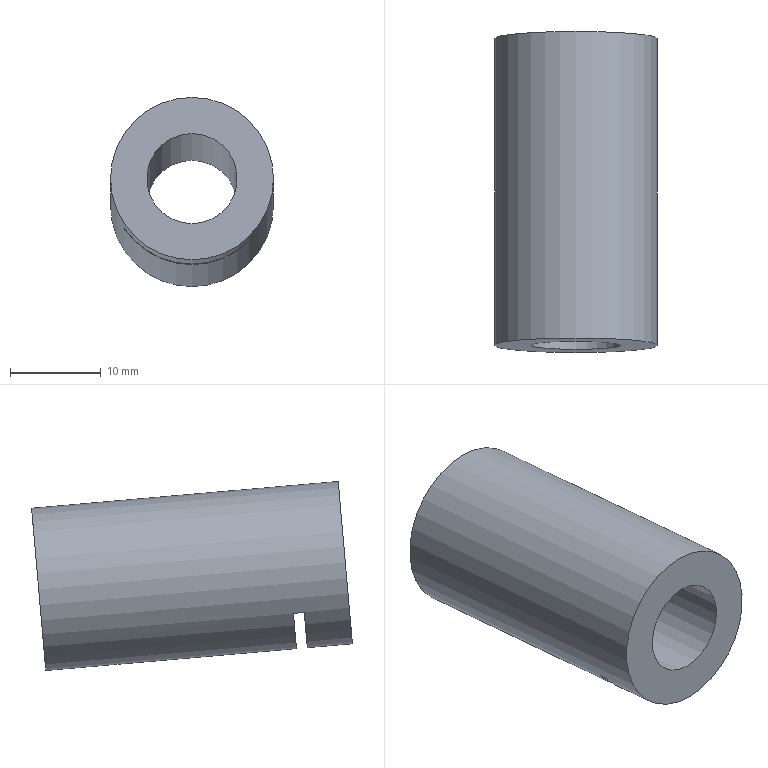Part | NX | features solid 2 | 1 solid | 7 faces | box 18 x 35.439 x 20.895 mm | volume 5933 mm3 | plane 5 | cylinder 2 | commonest cylinder face diameters 10 x1 18 x1
STEP:
#1=CARTESIAN_POINT('',(280.775,-80.843,-42.851));
#2=VERTEX_POINT('',#1);
#3=CARTESIAN_POINT('',(280.775,-81.278,-47.832));
#4=DIRECTION('',(0.,0.9962,-0.08716));
#5=DIRECTION('',(0.,0.08716,0.9962));
#6=AXIS2_PLACEMENT_3D('',#3,#4,#5);
#7=CIRCLE('',#6,5.);
#8=EDGE_CURVE('',#2,#2,#7,.T.);
#9=ORIENTED_EDGE('',*,*,#8,.F.);
#10=EDGE_LOOP('',(#9));
#11=FACE_BOUND('',#10,.T.);
#12=CARTESIAN_POINT('',(280.775,-80.494,-38.866));
#13=VERTEX_POINT('',#12);
#14=CARTESIAN_POINT('',(280.775,-81.278,-47.832));
#15=DIRECTION('',(0.,0.9962,-0.08716));
#16=DIRECTION('',(0.,0.08716,0.9962));
#17=AXIS2_PLACEMENT_3D('',#14,#15,#16);
#18=CIRCLE('',#17,9.);
#19=EDGE_CURVE('',#13,#13,#18,.F.);
#20=ORIENTED_EDGE('',*,*,#19,.F.);
#21=EDGE_LOOP('',(#20));
#22=FACE_BOUND('',#21,.T.);
#23=CARTESIAN_POINT('',(280.775,-81.278,-47.832));
#24=DIRECTION('',(0.,0.9962,-0.08716));
#25=DIRECTION('',(-1.,0.,0.));
#26=AXIS2_PLACEMENT_3D('',#23,#24,#25);
#27=PLANE('',#26);
#28=ADVANCED_FACE('',(#11,#22),#27,.T.);
#29=CARTESIAN_POINT('',(273.36,-110.612,-50.385));
#30=VERTEX_POINT('',#29);
#31=CARTESIAN_POINT('',(273.36,-109.417,-50.489));
#32=VERTEX_POINT('',#31);
#33=CARTESIAN_POINT('',(273.36,-57.017,-55.074));
#34=DIRECTION('',(0.,-0.9962,0.08716));
#35=VECTOR('',#34,1000.);
#36=LINE('',#33,#35);
#37=EDGE_CURVE('',#30,#32,#36,.F.);
#38=ORIENTED_EDGE('',*,*,#37,.F.);
#39=CARTESIAN_POINT('',(288.191,-110.612,-50.385));
#40=VERTEX_POINT('',#39);
#41=CARTESIAN_POINT('',(280.775,-110.168,-45.304));
#42=DIRECTION('',(0.,-0.9962,0.08716));
#43=DIRECTION('',(0.,-0.08716,-0.9962));
#44=AXIS2_PLACEMENT_3D('',#41,#42,#43);
#45=CIRCLE('',#44,9.);
#46=EDGE_CURVE('',#40,#30,#45,.F.);
#47=ORIENTED_EDGE('',*,*,#46,.F.);
#48=CARTESIAN_POINT('',(288.191,-109.417,-50.489));
#49=VERTEX_POINT('',#48);
#50=CARTESIAN_POINT('',(288.191,-57.017,-55.074));
#51=DIRECTION('',(0.,-0.9962,0.08716));
#52=VECTOR('',#51,1000.);
#53=LINE('',#50,#52);
#54=EDGE_CURVE('',#49,#40,#53,.T.);
#55=ORIENTED_EDGE('',*,*,#54,.F.);
#56=CARTESIAN_POINT('',(280.775,-108.973,-45.409));
#57=DIRECTION('',(0.,-0.9962,0.08716));
#58=DIRECTION('',(0.,-0.08716,-0.9962));
#59=AXIS2_PLACEMENT_3D('',#56,#57,#58);
#60=CIRCLE('',#59,9.);
#61=EDGE_CURVE('',#49,#32,#60,.F.);
#62=ORIENTED_EDGE('',*,*,#61,.T.);
#63=EDGE_LOOP('',(#38,#47,#55,#62));
#64=FACE_BOUND('',#63,.T.);
#65=ORIENTED_EDGE('',*,*,#19,.T.);
#66=EDGE_LOOP('',(#65));
#67=FACE_BOUND('',#66,.T.);
#68=CARTESIAN_POINT('',(280.775,-115.933,-53.834));
#69=VERTEX_POINT('',#68);
#70=CARTESIAN_POINT('',(280.775,-115.149,-44.868));
#71=DIRECTION('',(0.,-0.9962,0.08716));
#72=DIRECTION('',(0.,-0.08716,-0.9962));
#73=AXIS2_PLACEMENT_3D('',#70,#71,#72);
#74=CIRCLE('',#73,9.);
#75=EDGE_CURVE('',#69,#69,#74,.F.);
#76=ORIENTED_EDGE('',*,*,#75,.T.);
#77=EDGE_LOOP('',(#76));
#78=FACE_BOUND('',#77,.T.);
#79=CARTESIAN_POINT('',(280.775,-56.573,-49.993));
#80=DIRECTION('',(0.,-0.9962,0.08716));
#81=DIRECTION('',(1.,0.,0.));
#82=AXIS2_PLACEMENT_3D('',#79,#80,#81);
#83=CYLINDRICAL_SURFACE('',#82,9.);
#84=ADVANCED_FACE('',(#64,#67,#78),#83,.T.);
#85=CARTESIAN_POINT('',(280.775,-115.585,-49.849));
#86=VERTEX_POINT('',#85);
#87=CARTESIAN_POINT('',(280.775,-115.149,-44.868));
#88=DIRECTION('',(0.,-0.9962,0.08716));
#89=DIRECTION('',(0.,-0.08716,-0.9962));
#90=AXIS2_PLACEMENT_3D('',#87,#88,#89);
#91=CIRCLE('',#90,5.);
#92=EDGE_CURVE('',#86,#86,#91,.F.);
#93=ORIENTED_EDGE('',*,*,#92,.T.);
#94=EDGE_LOOP('',(#93));
#95=FACE_BOUND('',#94,.T.);
#96=ORIENTED_EDGE('',*,*,#75,.F.);
#97=EDGE_LOOP('',(#96));
#98=FACE_BOUND('',#97,.T.);
#99=CARTESIAN_POINT('',(280.775,-115.149,-44.868));
#100=DIRECTION('',(0.,-0.9962,0.08716));
#101=DIRECTION('',(-1.,0.,0.));
#102=AXIS2_PLACEMENT_3D('',#99,#100,#101);
#103=PLANE('',#102);
#104=ADVANCED_FACE('',(#95,#98),#103,.T.);
#105=ORIENTED_EDGE('',*,*,#8,.T.);
#106=EDGE_LOOP('',(#105));
#107=FACE_BOUND('',#106,.T.);
#108=ORIENTED_EDGE('',*,*,#92,.F.);
#109=EDGE_LOOP('',(#108));
#110=FACE_BOUND('',#109,.T.);
#111=CARTESIAN_POINT('',(280.775,-73.508,-48.512));
#112=DIRECTION('',(0.,-0.9962,0.08716));
#113=DIRECTION('',(0.,-0.08716,-0.9962));
#114=AXIS2_PLACEMENT_3D('',#111,#112,#113);
#115=CYLINDRICAL_SURFACE('',#114,5.);
#116=ADVANCED_FACE('',(#107,#110),#115,.F.);
#117=CARTESIAN_POINT('',(273.292,-109.417,-50.489));
#118=DIRECTION('',(-1.,0.,0.));
#119=VECTOR('',#118,1000.);
#120=LINE('',#117,#119);
#121=EDGE_CURVE('',#32,#49,#120,.F.);
#122=ORIENTED_EDGE('',*,*,#121,.F.);
#123=ORIENTED_EDGE('',*,*,#61,.F.);
#124=EDGE_LOOP('',(#122,#123));
#125=FACE_BOUND('',#124,.T.);
#126=CARTESIAN_POINT('',(273.292,-113.775,-100.299));
#127=DIRECTION('',(0.,-0.9962,0.08716));
#128=DIRECTION('',(0.,-0.08716,-0.9962));
#129=AXIS2_PLACEMENT_3D('',#126,#127,#128);
#130=PLANE('',#129);
#131=ADVANCED_FACE('',(#125),#130,.T.);
#132=ORIENTED_EDGE('',*,*,#46,.T.);
#133=CARTESIAN_POINT('',(273.292,-110.612,-50.385));
#134=DIRECTION('',(-1.,0.,0.));
#135=VECTOR('',#134,1000.);
#136=LINE('',#133,#135);
#137=EDGE_CURVE('',#30,#40,#136,.F.);
#138=ORIENTED_EDGE('',*,*,#137,.T.);
#139=EDGE_LOOP('',(#132,#138));
#140=FACE_BOUND('',#139,.T.);
#141=CARTESIAN_POINT('',(273.292,-114.97,-100.195));
#142=DIRECTION('',(0.,-0.9962,0.08716));
#143=DIRECTION('',(0.,-0.08716,-0.9962));
#144=AXIS2_PLACEMENT_3D('',#141,#142,#143);
#145=PLANE('',#144);
#146=ADVANCED_FACE('',(#140),#145,.F.);
#147=ORIENTED_EDGE('',*,*,#37,.T.);
#148=ORIENTED_EDGE('',*,*,#121,.T.);
#149=ORIENTED_EDGE('',*,*,#54,.T.);
#150=ORIENTED_EDGE('',*,*,#137,.F.);
#151=EDGE_LOOP('',(#147,#148,#149,#150));
#152=FACE_BOUND('',#151,.T.);
#153=CARTESIAN_POINT('',(273.292,-110.612,-50.385));
#154=DIRECTION('',(0.,0.08716,0.9962));
#155=DIRECTION('',(0.,0.9962,-0.08716));
#156=AXIS2_PLACEMENT_3D('',#153,#154,#155);
#157=PLANE('',#156);
#158=ADVANCED_FACE('',(#152),#157,.F.);
#159=CLOSED_SHELL('',(#28,#84,#104,#116,#131,#146,#158));
#160=MANIFOLD_SOLID_BREP('',#159);
#161=(LENGTH_UNIT()NAMED_UNIT(*)SI_UNIT(.MILLI.,.METRE.));
#162=UNCERTAINTY_MEASURE_WITH_UNIT(LENGTH_MEASURE(0.00001),#161,'','');
#163=(NAMED_UNIT(*)PLANE_ANGLE_UNIT()SI_UNIT($,.RADIAN.));
#164=(NAMED_UNIT(*)SI_UNIT($,.STERADIAN.)SOLID_ANGLE_UNIT());
#165=(GEOMETRIC_REPRESENTATION_CONTEXT(3)GLOBAL_UNCERTAINTY_ASSIGNED_CONTEXT((#162))GLOBAL_UNIT_ASSIGNED_CONTEXT((#161,#163,#164))REPRESENTATION_CONTEXT('',''));
#166=ADVANCED_BREP_SHAPE_REPRESENTATION('',(#160),#165);